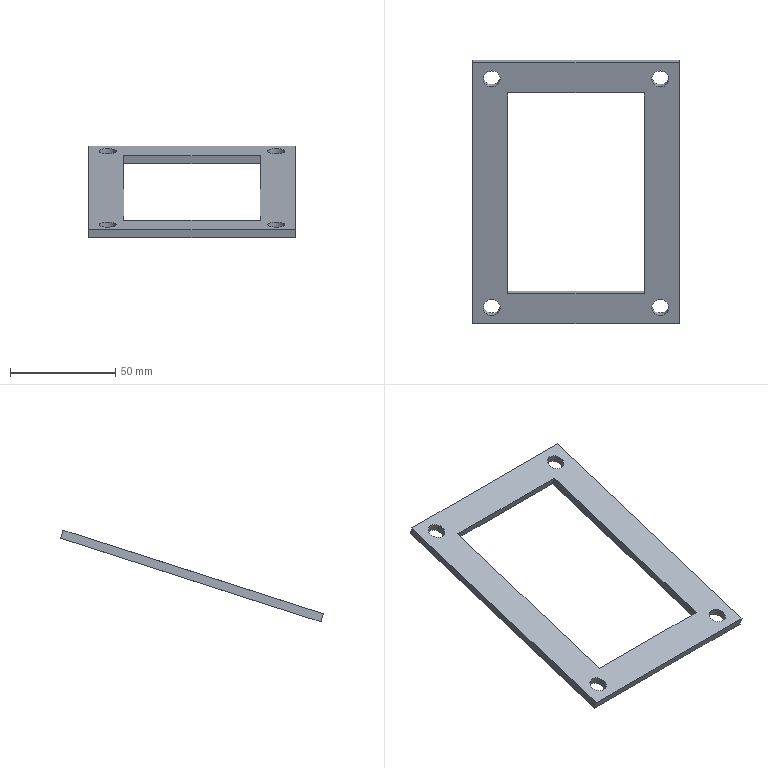Part | NX | features DATUM_CSYS 42, EXTRUDE 41, SKETCH 41, EXTRACT_DATUM_AXIS 38, EXTRACT_FACE 32, SIMPLE HOLE 20, EXTRACT_DATUM_PLANE 14, Instance Feature 13, DRAFT 9, EXTRACT_STRING 8, HOLE PACKAGE 7, FSET 6, Mirror Feature 5, BLEND 4, OFFSET_REGION 4, Pattern Feature 2, TRIM BODY 1 | 1 solid | 14 faces | box 98 x 124.993 x 43.573 mm | volume 24156 mm3 | plane 10 | cylinder 4 | commonest cylinder face diameters 8 x4
STEP:
#1=CARTESIAN_POINT('',(-49.,107.12,143.651));
#2=VERTEX_POINT('',#1);
#3=CARTESIAN_POINT('',(-49.,-16.649,103.887));
#4=VERTEX_POINT('',#3);
#5=CARTESIAN_POINT('',(-49.,107.12,143.651));
#6=DIRECTION('',(0.,-0.9521,-0.3059));
#7=VECTOR('',#6,1000.);
#8=LINE('',#5,#7);
#9=EDGE_CURVE('',#2,#4,#8,.T.);
#10=ORIENTED_EDGE('',*,*,#9,.F.);
#11=CARTESIAN_POINT('',(49.,107.12,143.651));
#12=VERTEX_POINT('',#11);
#13=CARTESIAN_POINT('',(49.,107.12,143.651));
#14=DIRECTION('',(-1.,0.,0.));
#15=VECTOR('',#14,1000.);
#16=LINE('',#13,#15);
#17=EDGE_CURVE('',#12,#2,#16,.T.);
#18=ORIENTED_EDGE('',*,*,#17,.F.);
#19=CARTESIAN_POINT('',(49.,-16.649,103.887));
#20=VERTEX_POINT('',#19);
#21=CARTESIAN_POINT('',(49.,-16.649,103.887));
#22=DIRECTION('',(0.,0.9521,0.3059));
#23=VECTOR('',#22,1000.);
#24=LINE('',#21,#23);
#25=EDGE_CURVE('',#20,#12,#24,.T.);
#26=ORIENTED_EDGE('',*,*,#25,.F.);
#27=CARTESIAN_POINT('',(-49.,-16.649,103.887));
#28=DIRECTION('',(1.,0.,0.));
#29=VECTOR('',#28,1000.);
#30=LINE('',#27,#29);
#31=EDGE_CURVE('',#4,#20,#30,.T.);
#32=ORIENTED_EDGE('',*,*,#31,.F.);
#33=EDGE_LOOP('',(#10,#18,#26,#32));
#34=FACE_BOUND('',#33,.T.);
#35=CARTESIAN_POINT('',(-40.,-5.224,107.557));
#36=VERTEX_POINT('',#35);
#37=CARTESIAN_POINT('',(-40.,-9.033,106.334));
#38=DIRECTION('',(0.,0.3059,-0.9521));
#39=DIRECTION('',(0.,0.9521,0.3059));
#40=AXIS2_PLACEMENT_3D('',#37,#38,#39);
#41=CIRCLE('',#40,4.);
#42=EDGE_CURVE('',#36,#36,#41,.F.);
#43=ORIENTED_EDGE('',*,*,#42,.T.);
#44=EDGE_LOOP('',(#43));
#45=FACE_BOUND('',#44,.T.);
#46=CARTESIAN_POINT('',(40.,-5.224,107.557));
#47=VERTEX_POINT('',#46);
#48=CARTESIAN_POINT('',(40.,-9.033,106.334));
#49=DIRECTION('',(0.,0.3059,-0.9521));
#50=DIRECTION('',(0.,0.9521,0.3059));
#51=AXIS2_PLACEMENT_3D('',#48,#49,#50);
#52=CIRCLE('',#51,4.);
#53=EDGE_CURVE('',#47,#47,#52,.T.);
#54=ORIENTED_EDGE('',*,*,#53,.F.);
#55=EDGE_LOOP('',(#54));
#56=FACE_BOUND('',#55,.T.);
#57=CARTESIAN_POINT('',(32.5,92.839,139.063));
#58=VERTEX_POINT('',#57);
#59=CARTESIAN_POINT('',(-32.5,92.839,139.063));
#60=VERTEX_POINT('',#59);
#61=CARTESIAN_POINT('',(-32.5,92.839,139.063));
#62=DIRECTION('',(-1.,0.,0.));
#63=VECTOR('',#62,1000.);
#64=LINE('',#61,#63);
#65=EDGE_CURVE('',#58,#60,#64,.T.);
#66=ORIENTED_EDGE('',*,*,#65,.T.);
#67=CARTESIAN_POINT('',(-32.5,-2.368,108.475));
#68=VERTEX_POINT('',#67);
#69=CARTESIAN_POINT('',(-32.5,-2.368,108.475));
#70=DIRECTION('',(0.,-0.9521,-0.3059));
#71=VECTOR('',#70,1000.);
#72=LINE('',#69,#71);
#73=EDGE_CURVE('',#60,#68,#72,.T.);
#74=ORIENTED_EDGE('',*,*,#73,.T.);
#75=CARTESIAN_POINT('',(32.5,-2.368,108.475));
#76=VERTEX_POINT('',#75);
#77=CARTESIAN_POINT('',(32.5,-2.368,108.475));
#78=DIRECTION('',(1.,0.,0.));
#79=VECTOR('',#78,1000.);
#80=LINE('',#77,#79);
#81=EDGE_CURVE('',#68,#76,#80,.T.);
#82=ORIENTED_EDGE('',*,*,#81,.T.);
#83=CARTESIAN_POINT('',(32.5,92.839,139.063));
#84=DIRECTION('',(0.,0.9521,0.3059));
#85=VECTOR('',#84,1000.);
#86=LINE('',#83,#85);
#87=EDGE_CURVE('',#76,#58,#86,.T.);
#88=ORIENTED_EDGE('',*,*,#87,.T.);
#89=EDGE_LOOP('',(#66,#74,#82,#88));
#90=FACE_BOUND('',#89,.T.);
#91=CARTESIAN_POINT('',(-40.,103.312,142.428));
#92=VERTEX_POINT('',#91);
#93=CARTESIAN_POINT('',(-40.,99.503,141.204));
#94=DIRECTION('',(0.,0.3059,-0.9521));
#95=DIRECTION('',(0.,0.9521,0.3059));
#96=AXIS2_PLACEMENT_3D('',#93,#94,#95);
#97=CIRCLE('',#96,4.);
#98=EDGE_CURVE('',#92,#92,#97,.T.);
#99=ORIENTED_EDGE('',*,*,#98,.F.);
#100=EDGE_LOOP('',(#99));
#101=FACE_BOUND('',#100,.T.);
#102=CARTESIAN_POINT('',(40.,103.312,142.428));
#103=VERTEX_POINT('',#102);
#104=CARTESIAN_POINT('',(40.,99.503,141.204));
#105=DIRECTION('',(0.,0.3059,-0.9521));
#106=DIRECTION('',(0.,0.9521,0.3059));
#107=AXIS2_PLACEMENT_3D('',#104,#105,#106);
#108=CIRCLE('',#107,4.);
#109=EDGE_CURVE('',#103,#103,#108,.F.);
#110=ORIENTED_EDGE('',*,*,#109,.T.);
#111=EDGE_LOOP('',(#110));
#112=FACE_BOUND('',#111,.T.);
#113=CARTESIAN_POINT('',(0.,45.235,123.769));
#114=DIRECTION('',(0.,0.3059,-0.9521));
#115=DIRECTION('',(0.,0.9521,0.3059));
#116=AXIS2_PLACEMENT_3D('',#113,#114,#115);
#117=PLANE('',#116);
#118=ADVANCED_FACE('',(#34,#45,#56,#90,#101,#112),#117,.T.);
#119=CARTESIAN_POINT('',(40.,102.088,146.236));
#120=VERTEX_POINT('',#119);
#121=CARTESIAN_POINT('',(40.,98.28,145.013));
#122=DIRECTION('',(0.,0.3059,-0.9521));
#123=DIRECTION('',(0.,0.9521,0.3059));
#124=AXIS2_PLACEMENT_3D('',#121,#122,#123);
#125=CIRCLE('',#124,4.);
#126=EDGE_CURVE('',#120,#120,#125,.T.);
#127=ORIENTED_EDGE('',*,*,#126,.F.);
#128=EDGE_LOOP('',(#127));
#129=FACE_BOUND('',#128,.T.);
#130=ORIENTED_EDGE('',*,*,#109,.F.);
#131=EDGE_LOOP('',(#130));
#132=FACE_BOUND('',#131,.T.);
#133=CARTESIAN_POINT('',(40.,98.28,145.013));
#134=DIRECTION('',(0.,0.3059,-0.9521));
#135=DIRECTION('',(0.,0.9521,0.3059));
#136=AXIS2_PLACEMENT_3D('',#133,#134,#135);
#137=CYLINDRICAL_SURFACE('',#136,4.);
#138=ADVANCED_FACE('',(#129,#132),#137,.F.);
#139=CARTESIAN_POINT('',(-40.,102.088,146.236));
#140=VERTEX_POINT('',#139);
#141=CARTESIAN_POINT('',(-40.,98.28,145.013));
#142=DIRECTION('',(0.,-0.3059,0.9521));
#143=DIRECTION('',(0.,0.9521,0.3059));
#144=AXIS2_PLACEMENT_3D('',#141,#142,#143);
#145=CIRCLE('',#144,4.);
#146=EDGE_CURVE('',#140,#140,#145,.T.);
#147=ORIENTED_EDGE('',*,*,#146,.T.);
#148=EDGE_LOOP('',(#147));
#149=FACE_BOUND('',#148,.T.);
#150=ORIENTED_EDGE('',*,*,#98,.T.);
#151=EDGE_LOOP('',(#150));
#152=FACE_BOUND('',#151,.T.);
#153=CARTESIAN_POINT('',(-40.,98.28,145.013));
#154=DIRECTION('',(0.,0.3059,-0.9521));
#155=DIRECTION('',(0.,0.9521,0.3059));
#156=AXIS2_PLACEMENT_3D('',#153,#154,#155);
#157=CYLINDRICAL_SURFACE('',#156,4.);
#158=ADVANCED_FACE('',(#149,#152),#157,.F.);
#159=ORIENTED_EDGE('',*,*,#73,.F.);
#160=CARTESIAN_POINT('',(-32.5,91.615,142.871));
#161=VERTEX_POINT('',#160);
#162=CARTESIAN_POINT('',(-32.5,91.615,142.871));
#163=DIRECTION('',(0.,0.3059,-0.9521));
#164=VECTOR('',#163,1000.);
#165=LINE('',#162,#164);
#166=EDGE_CURVE('',#161,#60,#165,.T.);
#167=ORIENTED_EDGE('',*,*,#166,.F.);
#168=CARTESIAN_POINT('',(-32.5,-3.592,112.283));
#169=VERTEX_POINT('',#168);
#170=CARTESIAN_POINT('',(-32.5,-3.592,112.283));
#171=DIRECTION('',(0.,0.9521,0.3059));
#172=VECTOR('',#171,1000.);
#173=LINE('',#170,#172);
#174=EDGE_CURVE('',#169,#161,#173,.T.);
#175=ORIENTED_EDGE('',*,*,#174,.F.);
#176=CARTESIAN_POINT('',(-32.5,-3.592,112.283));
#177=DIRECTION('',(0.,0.3059,-0.9521));
#178=VECTOR('',#177,1000.);
#179=LINE('',#176,#178);
#180=EDGE_CURVE('',#169,#68,#179,.T.);
#181=ORIENTED_EDGE('',*,*,#180,.T.);
#182=EDGE_LOOP('',(#159,#167,#175,#181));
#183=FACE_BOUND('',#182,.T.);
#184=CARTESIAN_POINT('',(-32.5,-3.592,112.283));
#185=DIRECTION('',(-1.,0.,0.));
#186=DIRECTION('',(0.,0.,1.));
#187=AXIS2_PLACEMENT_3D('',#184,#185,#186);
#188=PLANE('',#187);
#189=ADVANCED_FACE('',(#183),#188,.F.);
#190=ORIENTED_EDGE('',*,*,#65,.F.);
#191=CARTESIAN_POINT('',(32.5,91.615,142.871));
#192=VERTEX_POINT('',#191);
#193=CARTESIAN_POINT('',(32.5,91.615,142.871));
#194=DIRECTION('',(0.,0.3059,-0.9521));
#195=VECTOR('',#194,1000.);
#196=LINE('',#193,#195);
#197=EDGE_CURVE('',#192,#58,#196,.T.);
#198=ORIENTED_EDGE('',*,*,#197,.F.);
#199=CARTESIAN_POINT('',(-32.5,91.615,142.871));
#200=DIRECTION('',(1.,0.,0.));
#201=VECTOR('',#200,1000.);
#202=LINE('',#199,#201);
#203=EDGE_CURVE('',#161,#192,#202,.T.);
#204=ORIENTED_EDGE('',*,*,#203,.F.);
#205=ORIENTED_EDGE('',*,*,#166,.T.);
#206=EDGE_LOOP('',(#190,#198,#204,#205));
#207=FACE_BOUND('',#206,.T.);
#208=CARTESIAN_POINT('',(-32.5,91.615,142.871));
#209=DIRECTION('',(0.,0.9521,0.3059));
#210=DIRECTION('',(0.,-0.3059,0.9521));
#211=AXIS2_PLACEMENT_3D('',#208,#209,#210);
#212=PLANE('',#211);
#213=ADVANCED_FACE('',(#207),#212,.F.);
#214=ORIENTED_EDGE('',*,*,#87,.F.);
#215=CARTESIAN_POINT('',(32.5,-3.592,112.283));
#216=VERTEX_POINT('',#215);
#217=CARTESIAN_POINT('',(32.5,-3.592,112.283));
#218=DIRECTION('',(0.,0.3059,-0.9521));
#219=VECTOR('',#218,1000.);
#220=LINE('',#217,#219);
#221=EDGE_CURVE('',#216,#76,#220,.T.);
#222=ORIENTED_EDGE('',*,*,#221,.F.);
#223=CARTESIAN_POINT('',(32.5,91.615,142.871));
#224=DIRECTION('',(0.,-0.9521,-0.3059));
#225=VECTOR('',#224,1000.);
#226=LINE('',#223,#225);
#227=EDGE_CURVE('',#192,#216,#226,.T.);
#228=ORIENTED_EDGE('',*,*,#227,.F.);
#229=ORIENTED_EDGE('',*,*,#197,.T.);
#230=EDGE_LOOP('',(#214,#222,#228,#229));
#231=FACE_BOUND('',#230,.T.);
#232=CARTESIAN_POINT('',(32.5,91.615,142.871));
#233=DIRECTION('',(1.,0.,0.));
#234=DIRECTION('',(0.,0.,-1.));
#235=AXIS2_PLACEMENT_3D('',#232,#233,#234);
#236=PLANE('',#235);
#237=ADVANCED_FACE('',(#231),#236,.F.);
#238=CARTESIAN_POINT('',(-40.,-14.064,108.918));
#239=VERTEX_POINT('',#238);
#240=CARTESIAN_POINT('',(-40.,-10.256,110.142));
#241=DIRECTION('',(0.,0.3059,-0.9521));
#242=DIRECTION('',(0.,-0.9521,-0.3059));
#243=AXIS2_PLACEMENT_3D('',#240,#241,#242);
#244=CIRCLE('',#243,4.);
#245=EDGE_CURVE('',#239,#239,#244,.T.);
#246=ORIENTED_EDGE('',*,*,#245,.F.);
#247=EDGE_LOOP('',(#246));
#248=FACE_BOUND('',#247,.T.);
#249=ORIENTED_EDGE('',*,*,#42,.F.);
#250=EDGE_LOOP('',(#249));
#251=FACE_BOUND('',#250,.T.);
#252=CARTESIAN_POINT('',(-40.,-10.256,110.142));
#253=DIRECTION('',(0.,0.3059,-0.9521));
#254=DIRECTION('',(0.,0.9521,0.3059));
#255=AXIS2_PLACEMENT_3D('',#252,#253,#254);
#256=CYLINDRICAL_SURFACE('',#255,4.);
#257=ADVANCED_FACE('',(#248,#251),#256,.F.);
#258=CARTESIAN_POINT('',(40.,-14.064,108.918));
#259=VERTEX_POINT('',#258);
#260=CARTESIAN_POINT('',(40.,-10.256,110.142));
#261=DIRECTION('',(0.,-0.3059,0.9521));
#262=DIRECTION('',(0.,-0.9521,-0.3059));
#263=AXIS2_PLACEMENT_3D('',#260,#261,#262);
#264=CIRCLE('',#263,4.);
#265=EDGE_CURVE('',#259,#259,#264,.T.);
#266=ORIENTED_EDGE('',*,*,#265,.T.);
#267=EDGE_LOOP('',(#266));
#268=FACE_BOUND('',#267,.T.);
#269=ORIENTED_EDGE('',*,*,#53,.T.);
#270=EDGE_LOOP('',(#269));
#271=FACE_BOUND('',#270,.T.);
#272=CARTESIAN_POINT('',(40.,-10.256,110.142));
#273=DIRECTION('',(0.,0.3059,-0.9521));
#274=DIRECTION('',(0.,0.9521,0.3059));
#275=AXIS2_PLACEMENT_3D('',#272,#273,#274);
#276=CYLINDRICAL_SURFACE('',#275,4.);
#277=ADVANCED_FACE('',(#268,#271),#276,.F.);
#278=ORIENTED_EDGE('',*,*,#81,.F.);
#279=ORIENTED_EDGE('',*,*,#180,.F.);
#280=CARTESIAN_POINT('',(32.5,-3.592,112.283));
#281=DIRECTION('',(-1.,0.,0.));
#282=VECTOR('',#281,1000.);
#283=LINE('',#280,#282);
#284=EDGE_CURVE('',#216,#169,#283,.T.);
#285=ORIENTED_EDGE('',*,*,#284,.F.);
#286=ORIENTED_EDGE('',*,*,#221,.T.);
#287=EDGE_LOOP('',(#278,#279,#285,#286));
#288=FACE_BOUND('',#287,.T.);
#289=CARTESIAN_POINT('',(32.5,-3.592,112.283));
#290=DIRECTION('',(0.,-0.9521,-0.3059));
#291=DIRECTION('',(0.,0.3059,-0.9521));
#292=AXIS2_PLACEMENT_3D('',#289,#290,#291);
#293=PLANE('',#292);
#294=ADVANCED_FACE('',(#288),#293,.F.);
#295=ORIENTED_EDGE('',*,*,#9,.T.);
#296=CARTESIAN_POINT('',(-49.,-17.873,107.695));
#297=VERTEX_POINT('',#296);
#298=CARTESIAN_POINT('',(-49.,-17.873,107.695));
#299=DIRECTION('',(0.,0.3059,-0.9521));
#300=VECTOR('',#299,1000.);
#301=LINE('',#298,#300);
#302=EDGE_CURVE('',#297,#4,#301,.T.);
#303=ORIENTED_EDGE('',*,*,#302,.F.);
#304=CARTESIAN_POINT('',(-49.,105.896,147.46));
#305=VERTEX_POINT('',#304);
#306=CARTESIAN_POINT('',(-49.,105.896,147.46));
#307=DIRECTION('',(0.,-0.9521,-0.3059));
#308=VECTOR('',#307,1000.);
#309=LINE('',#306,#308);
#310=EDGE_CURVE('',#305,#297,#309,.T.);
#311=ORIENTED_EDGE('',*,*,#310,.F.);
#312=CARTESIAN_POINT('',(-49.,105.896,147.46));
#313=DIRECTION('',(0.,0.3059,-0.9521));
#314=VECTOR('',#313,1000.);
#315=LINE('',#312,#314);
#316=EDGE_CURVE('',#305,#2,#315,.T.);
#317=ORIENTED_EDGE('',*,*,#316,.T.);
#318=EDGE_LOOP('',(#295,#303,#311,#317));
#319=FACE_BOUND('',#318,.T.);
#320=CARTESIAN_POINT('',(-49.,105.896,147.46));
#321=DIRECTION('',(1.,0.,0.));
#322=DIRECTION('',(0.,0.,-1.));
#323=AXIS2_PLACEMENT_3D('',#320,#321,#322);
#324=PLANE('',#323);
#325=ADVANCED_FACE('',(#319),#324,.F.);
#326=ORIENTED_EDGE('',*,*,#31,.T.);
#327=CARTESIAN_POINT('',(49.,-17.873,107.695));
#328=VERTEX_POINT('',#327);
#329=CARTESIAN_POINT('',(49.,-17.873,107.695));
#330=DIRECTION('',(0.,0.3059,-0.9521));
#331=VECTOR('',#330,1000.);
#332=LINE('',#329,#331);
#333=EDGE_CURVE('',#328,#20,#332,.T.);
#334=ORIENTED_EDGE('',*,*,#333,.F.);
#335=CARTESIAN_POINT('',(-49.,-17.873,107.695));
#336=DIRECTION('',(1.,0.,0.));
#337=VECTOR('',#336,1000.);
#338=LINE('',#335,#337);
#339=EDGE_CURVE('',#297,#328,#338,.T.);
#340=ORIENTED_EDGE('',*,*,#339,.F.);
#341=ORIENTED_EDGE('',*,*,#302,.T.);
#342=EDGE_LOOP('',(#326,#334,#340,#341));
#343=FACE_BOUND('',#342,.T.);
#344=CARTESIAN_POINT('',(-49.,-17.873,107.695));
#345=DIRECTION('',(0.,0.9521,0.3059));
#346=DIRECTION('',(0.,-0.3059,0.9521));
#347=AXIS2_PLACEMENT_3D('',#344,#345,#346);
#348=PLANE('',#347);
#349=ADVANCED_FACE('',(#343),#348,.F.);
#350=ORIENTED_EDGE('',*,*,#25,.T.);
#351=CARTESIAN_POINT('',(49.,105.896,147.46));
#352=VERTEX_POINT('',#351);
#353=CARTESIAN_POINT('',(49.,105.896,147.46));
#354=DIRECTION('',(0.,0.3059,-0.9521));
#355=VECTOR('',#354,1000.);
#356=LINE('',#353,#355);
#357=EDGE_CURVE('',#352,#12,#356,.T.);
#358=ORIENTED_EDGE('',*,*,#357,.F.);
#359=CARTESIAN_POINT('',(49.,-17.873,107.695));
#360=DIRECTION('',(0.,0.9521,0.3059));
#361=VECTOR('',#360,1000.);
#362=LINE('',#359,#361);
#363=EDGE_CURVE('',#328,#352,#362,.T.);
#364=ORIENTED_EDGE('',*,*,#363,.F.);
#365=ORIENTED_EDGE('',*,*,#333,.T.);
#366=EDGE_LOOP('',(#350,#358,#364,#365));
#367=FACE_BOUND('',#366,.T.);
#368=CARTESIAN_POINT('',(49.,-17.873,107.695));
#369=DIRECTION('',(-1.,0.,0.));
#370=DIRECTION('',(0.,0.,1.));
#371=AXIS2_PLACEMENT_3D('',#368,#369,#370);
#372=PLANE('',#371);
#373=ADVANCED_FACE('',(#367),#372,.F.);
#374=ORIENTED_EDGE('',*,*,#17,.T.);
#375=ORIENTED_EDGE('',*,*,#316,.F.);
#376=CARTESIAN_POINT('',(49.,105.896,147.46));
#377=DIRECTION('',(-1.,0.,0.));
#378=VECTOR('',#377,1000.);
#379=LINE('',#376,#378);
#380=EDGE_CURVE('',#352,#305,#379,.T.);
#381=ORIENTED_EDGE('',*,*,#380,.F.);
#382=ORIENTED_EDGE('',*,*,#357,.T.);
#383=EDGE_LOOP('',(#374,#375,#381,#382));
#384=FACE_BOUND('',#383,.T.);
#385=CARTESIAN_POINT('',(49.,105.896,147.46));
#386=DIRECTION('',(0.,-0.9521,-0.3059));
#387=DIRECTION('',(0.,0.3059,-0.9521));
#388=AXIS2_PLACEMENT_3D('',#385,#386,#387);
#389=PLANE('',#388);
#390=ADVANCED_FACE('',(#384),#389,.F.);
#391=ORIENTED_EDGE('',*,*,#310,.T.);
#392=ORIENTED_EDGE('',*,*,#339,.T.);
#393=ORIENTED_EDGE('',*,*,#363,.T.);
#394=ORIENTED_EDGE('',*,*,#380,.T.);
#395=EDGE_LOOP('',(#391,#392,#393,#394));
#396=FACE_BOUND('',#395,.T.);
#397=ORIENTED_EDGE('',*,*,#126,.T.);
#398=EDGE_LOOP('',(#397));
#399=FACE_BOUND('',#398,.T.);
#400=ORIENTED_EDGE('',*,*,#265,.F.);
#401=EDGE_LOOP('',(#400));
#402=FACE_BOUND('',#401,.T.);
#403=ORIENTED_EDGE('',*,*,#146,.F.);
#404=EDGE_LOOP('',(#403));
#405=FACE_BOUND('',#404,.T.);
#406=ORIENTED_EDGE('',*,*,#245,.T.);
#407=EDGE_LOOP('',(#406));
#408=FACE_BOUND('',#407,.T.);
#409=ORIENTED_EDGE('',*,*,#174,.T.);
#410=ORIENTED_EDGE('',*,*,#203,.T.);
#411=ORIENTED_EDGE('',*,*,#227,.T.);
#412=ORIENTED_EDGE('',*,*,#284,.T.);
#413=EDGE_LOOP('',(#409,#410,#411,#412));
#414=FACE_BOUND('',#413,.T.);
#415=CARTESIAN_POINT('',(40.,98.28,145.013));
#416=DIRECTION('',(0.,0.3059,-0.9521));
#417=DIRECTION('',(0.,0.9521,0.3059));
#418=AXIS2_PLACEMENT_3D('',#415,#416,#417);
#419=PLANE('',#418);
#420=ADVANCED_FACE('',(#396,#399,#402,#405,#408,#414),#419,.F.);
#421=CLOSED_SHELL('',(#118,#138,#158,#189,#213,#237,#257,#277,#294,#325,#349,#373,#390,#420));
#422=MANIFOLD_SOLID_BREP('',#421);
#423=(LENGTH_UNIT()NAMED_UNIT(*)SI_UNIT(.MILLI.,.METRE.));
#424=UNCERTAINTY_MEASURE_WITH_UNIT(LENGTH_MEASURE(0.00001),#423,'','');
#425=(NAMED_UNIT(*)PLANE_ANGLE_UNIT()SI_UNIT($,.RADIAN.));
#426=(NAMED_UNIT(*)SI_UNIT($,.STERADIAN.)SOLID_ANGLE_UNIT());
#427=(GEOMETRIC_REPRESENTATION_CONTEXT(3)GLOBAL_UNCERTAINTY_ASSIGNED_CONTEXT((#424))GLOBAL_UNIT_ASSIGNED_CONTEXT((#423,#425,#426))REPRESENTATION_CONTEXT('',''));
#428=ADVANCED_BREP_SHAPE_REPRESENTATION('',(#422),#427);